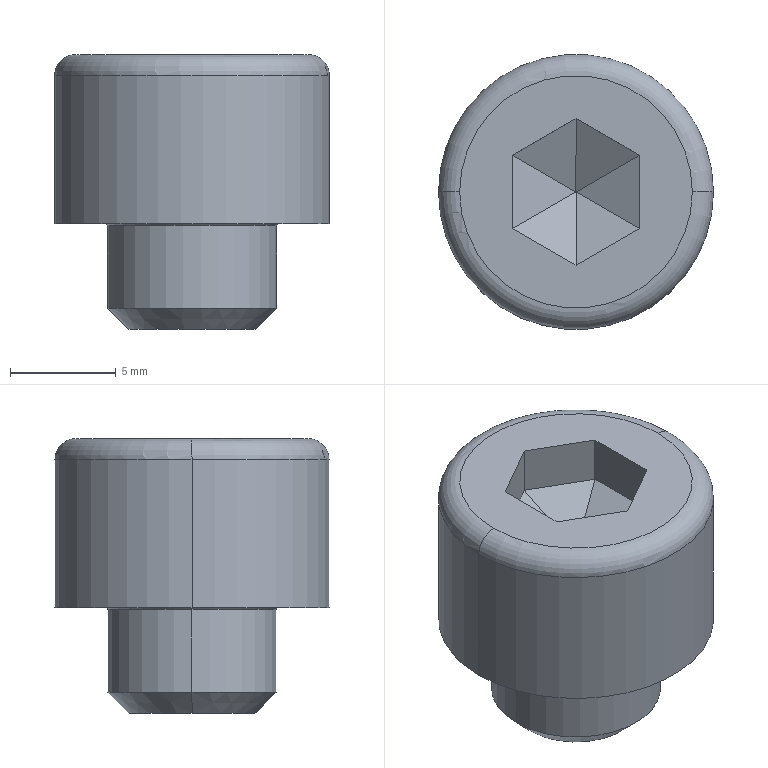Part | STEP file | Socket head cap screw M8x5 | 1 solid | 26 faces | box 13 x 13 x 13 mm | volume 1204 mm3 | plane 16 | torus 4 | cylinder 4 | cone 2 | commonest cylinder face diameters 8 x2 13 x2
STEP:
#1=CARTESIAN_POINT('',(-4.1,0.,0.));
#2=VERTEX_POINT('',#1);
#3=CARTESIAN_POINT('',(4.1,0.,0.));
#4=VERTEX_POINT('',#3);
#5=CARTESIAN_POINT('',(0.,0.,0.));
#6=DIRECTION('',(0.,0.,1.));
#7=DIRECTION('',(1.,0.,0.));
#8=AXIS2_PLACEMENT_3D('',#5,#6,#7);
#9=CIRCLE('',#8,4.1);
#10=EDGE_CURVE('',#2,#4,#9,.T.);
#11=ORIENTED_EDGE('',*,*,#10,.F.);
#12=CARTESIAN_POINT('',(-4.,0.,-0.1));
#13=VERTEX_POINT('',#12);
#14=CARTESIAN_POINT('',(-4.1,0.,-0.1));
#15=DIRECTION('',(0.,1.,0.));
#16=DIRECTION('',(-1.,0.,0.));
#17=AXIS2_PLACEMENT_3D('',#14,#15,#16);
#18=CIRCLE('',#17,0.1);
#19=EDGE_CURVE('',#2,#13,#18,.T.);
#20=ORIENTED_EDGE('',*,*,#19,.T.);
#21=CARTESIAN_POINT('',(4.,0.,-0.1));
#22=VERTEX_POINT('',#21);
#23=CARTESIAN_POINT('',(0.,0.,-0.1));
#24=DIRECTION('',(0.,0.,-1.));
#25=DIRECTION('',(1.,0.,0.));
#26=AXIS2_PLACEMENT_3D('',#23,#24,#25);
#27=CIRCLE('',#26,4.);
#28=EDGE_CURVE('',#22,#13,#27,.T.);
#29=ORIENTED_EDGE('',*,*,#28,.F.);
#30=CARTESIAN_POINT('',(4.1,0.,-0.1));
#31=DIRECTION('',(0.,-1.,0.));
#32=DIRECTION('',(0.,0.,-1.));
#33=AXIS2_PLACEMENT_3D('',#30,#31,#32);
#34=CIRCLE('',#33,0.1);
#35=EDGE_CURVE('',#4,#22,#34,.T.);
#36=ORIENTED_EDGE('',*,*,#35,.F.);
#37=EDGE_LOOP('',(#11,#20,#29,#36));
#38=FACE_OUTER_BOUND('',#37,.T.);
#39=CARTESIAN_POINT('',(0.,0.,-0.1));
#40=DIRECTION('',(0.,0.,1.));
#41=DIRECTION('',(1.,0.,0.));
#42=AXIS2_PLACEMENT_3D('',#39,#40,#41);
#43=TOROIDAL_SURFACE('',#42,4.1,0.1);
#44=ADVANCED_FACE('',(#38),#43,.F.);
#45=CARTESIAN_POINT('',(-6.5,0.,7.));
#46=VERTEX_POINT('',#45);
#47=CARTESIAN_POINT('',(6.5,0.,7.));
#48=VERTEX_POINT('',#47);
#49=CARTESIAN_POINT('',(0.,0.,7.));
#50=DIRECTION('',(0.,0.,-1.));
#51=DIRECTION('',(1.,0.,0.));
#52=AXIS2_PLACEMENT_3D('',#49,#50,#51);
#53=CIRCLE('',#52,6.5);
#54=EDGE_CURVE('',#46,#48,#53,.T.);
#55=ORIENTED_EDGE('',*,*,#54,.F.);
#56=CARTESIAN_POINT('',(-5.5,0.,8.));
#57=VERTEX_POINT('',#56);
#58=CARTESIAN_POINT('',(-5.5,0.,7.));
#59=DIRECTION('',(0.,1.,0.));
#60=DIRECTION('',(-1.,0.,0.));
#61=AXIS2_PLACEMENT_3D('',#58,#59,#60);
#62=CIRCLE('',#61,1.);
#63=EDGE_CURVE('',#46,#57,#62,.T.);
#64=ORIENTED_EDGE('',*,*,#63,.T.);
#65=CARTESIAN_POINT('',(5.5,0.,8.));
#66=VERTEX_POINT('',#65);
#67=CARTESIAN_POINT('',(0.,0.,8.));
#68=DIRECTION('',(0.,0.,1.));
#69=DIRECTION('',(1.,0.,0.));
#70=AXIS2_PLACEMENT_3D('',#67,#68,#69);
#71=CIRCLE('',#70,5.5);
#72=EDGE_CURVE('',#66,#57,#71,.T.);
#73=ORIENTED_EDGE('',*,*,#72,.F.);
#74=CARTESIAN_POINT('',(5.5,0.,7.));
#75=DIRECTION('',(0.,-1.,0.));
#76=DIRECTION('',(0.,0.,-1.));
#77=AXIS2_PLACEMENT_3D('',#74,#75,#76);
#78=CIRCLE('',#77,1.);
#79=EDGE_CURVE('',#48,#66,#78,.T.);
#80=ORIENTED_EDGE('',*,*,#79,.F.);
#81=EDGE_LOOP('',(#55,#64,#73,#80));
#82=FACE_OUTER_BOUND('',#81,.T.);
#83=CARTESIAN_POINT('',(0.,0.,7.));
#84=DIRECTION('',(0.,0.,1.));
#85=DIRECTION('',(1.,0.,0.));
#86=AXIS2_PLACEMENT_3D('',#83,#84,#85);
#87=TOROIDAL_SURFACE('',#86,5.5,1.);
#88=ADVANCED_FACE('',(#82),#87,.T.);
#89=CARTESIAN_POINT('',(-3.,0.,-5.));
#90=VERTEX_POINT('',#89);
#91=CARTESIAN_POINT('',(3.,0.,-5.));
#92=VERTEX_POINT('',#91);
#93=CARTESIAN_POINT('',(0.,0.,-5.));
#94=DIRECTION('',(0.,0.,-1.));
#95=DIRECTION('',(-1.,0.,0.));
#96=AXIS2_PLACEMENT_3D('',#93,#94,#95);
#97=CIRCLE('',#96,3.);
#98=EDGE_CURVE('',#90,#92,#97,.T.);
#99=ORIENTED_EDGE('',*,*,#98,.F.);
#100=CARTESIAN_POINT('',(-4.,0.,-4.));
#101=VERTEX_POINT('',#100);
#102=CARTESIAN_POINT('',(-3.,0.,-5.));
#103=DIRECTION('',(-0.7071,0.,0.7071));
#104=VECTOR('',#103,1000.);
#105=LINE('',#102,#104);
#106=EDGE_CURVE('',#90,#101,#105,.T.);
#107=ORIENTED_EDGE('',*,*,#106,.T.);
#108=CARTESIAN_POINT('',(4.,0.,-4.));
#109=VERTEX_POINT('',#108);
#110=CARTESIAN_POINT('',(0.,0.,-4.));
#111=DIRECTION('',(0.,0.,1.));
#112=DIRECTION('',(-1.,0.,0.));
#113=AXIS2_PLACEMENT_3D('',#110,#111,#112);
#114=CIRCLE('',#113,4.);
#115=EDGE_CURVE('',#109,#101,#114,.T.);
#116=ORIENTED_EDGE('',*,*,#115,.F.);
#117=CARTESIAN_POINT('',(3.,0.,-5.));
#118=DIRECTION('',(0.7071,0.,0.7071));
#119=VECTOR('',#118,1000.);
#120=LINE('',#117,#119);
#121=EDGE_CURVE('',#92,#109,#120,.T.);
#122=ORIENTED_EDGE('',*,*,#121,.F.);
#123=EDGE_LOOP('',(#99,#107,#116,#122));
#124=FACE_OUTER_BOUND('',#123,.T.);
#125=CARTESIAN_POINT('',(0.,0.,-5.));
#126=DIRECTION('',(0.,0.,1.));
#127=DIRECTION('',(1.,0.,0.));
#128=AXIS2_PLACEMENT_3D('',#125,#126,#127);
#129=CONICAL_SURFACE('',#128,3.,0.7854);
#130=ADVANCED_FACE('',(#124),#129,.T.);
#131=ORIENTED_EDGE('',*,*,#115,.T.);
#132=CARTESIAN_POINT('',(-4.,0.,-5.));
#133=DIRECTION('',(0.,0.,1.));
#134=VECTOR('',#133,1000.);
#135=LINE('',#132,#134);
#136=EDGE_CURVE('',#101,#13,#135,.T.);
#137=ORIENTED_EDGE('',*,*,#136,.T.);
#138=CARTESIAN_POINT('',(0.,0.,-0.1));
#139=DIRECTION('',(0.,0.,-1.));
#140=DIRECTION('',(1.,0.,0.));
#141=AXIS2_PLACEMENT_3D('',#138,#139,#140);
#142=CIRCLE('',#141,4.);
#143=EDGE_CURVE('',#13,#22,#142,.T.);
#144=ORIENTED_EDGE('',*,*,#143,.T.);
#145=CARTESIAN_POINT('',(4.,0.,-5.));
#146=DIRECTION('',(0.,0.,1.));
#147=VECTOR('',#146,1000.);
#148=LINE('',#145,#147);
#149=EDGE_CURVE('',#109,#22,#148,.T.);
#150=ORIENTED_EDGE('',*,*,#149,.F.);
#151=EDGE_LOOP('',(#131,#137,#144,#150));
#152=FACE_OUTER_BOUND('',#151,.T.);
#153=CARTESIAN_POINT('',(0.,0.,-5.));
#154=DIRECTION('',(0.,0.,1.));
#155=DIRECTION('',(1.,0.,0.));
#156=AXIS2_PLACEMENT_3D('',#153,#154,#155);
#157=CYLINDRICAL_SURFACE('',#156,4.);
#158=ADVANCED_FACE('',(#152),#157,.T.);
#159=ORIENTED_EDGE('',*,*,#54,.T.);
#160=CARTESIAN_POINT('',(6.5,0.,0.));
#161=VERTEX_POINT('',#160);
#162=CARTESIAN_POINT('',(6.5,0.,8.));
#163=DIRECTION('',(0.,0.,-1.));
#164=VECTOR('',#163,1000.);
#165=LINE('',#162,#164);
#166=EDGE_CURVE('',#48,#161,#165,.T.);
#167=ORIENTED_EDGE('',*,*,#166,.T.);
#168=CARTESIAN_POINT('',(-6.5,0.,0.));
#169=VERTEX_POINT('',#168);
#170=CARTESIAN_POINT('',(0.,0.,0.));
#171=DIRECTION('',(0.,0.,1.));
#172=DIRECTION('',(1.,0.,0.));
#173=AXIS2_PLACEMENT_3D('',#170,#171,#172);
#174=CIRCLE('',#173,6.5);
#175=EDGE_CURVE('',#161,#169,#174,.T.);
#176=ORIENTED_EDGE('',*,*,#175,.T.);
#177=CARTESIAN_POINT('',(-6.5,0.,8.));
#178=DIRECTION('',(0.,0.,-1.));
#179=VECTOR('',#178,1000.);
#180=LINE('',#177,#179);
#181=EDGE_CURVE('',#46,#169,#180,.T.);
#182=ORIENTED_EDGE('',*,*,#181,.F.);
#183=EDGE_LOOP('',(#159,#167,#176,#182));
#184=FACE_OUTER_BOUND('',#183,.T.);
#185=CARTESIAN_POINT('',(0.,0.,8.));
#186=DIRECTION('',(0.,0.,-1.));
#187=DIRECTION('',(-1.,0.,0.));
#188=AXIS2_PLACEMENT_3D('',#185,#186,#187);
#189=CYLINDRICAL_SURFACE('',#188,6.5);
#190=ADVANCED_FACE('',(#184),#189,.T.);
#191=CARTESIAN_POINT('',(0.,0.,0.));
#192=DIRECTION('',(0.,0.,1.));
#193=DIRECTION('',(1.,0.,0.));
#194=AXIS2_PLACEMENT_3D('',#191,#192,#193);
#195=CIRCLE('',#194,4.1);
#196=EDGE_CURVE('',#4,#2,#195,.T.);
#197=ORIENTED_EDGE('',*,*,#196,.T.);
#198=ORIENTED_EDGE('',*,*,#10,.T.);
#199=EDGE_LOOP('',(#197,#198));
#200=FACE_BOUND('',#199,.T.);
#201=CARTESIAN_POINT('',(0.,0.,0.));
#202=DIRECTION('',(0.,0.,1.));
#203=DIRECTION('',(1.,0.,0.));
#204=AXIS2_PLACEMENT_3D('',#201,#202,#203);
#205=CIRCLE('',#204,6.5);
#206=EDGE_CURVE('',#169,#161,#205,.T.);
#207=ORIENTED_EDGE('',*,*,#206,.F.);
#208=ORIENTED_EDGE('',*,*,#175,.F.);
#209=EDGE_LOOP('',(#207,#208));
#210=FACE_OUTER_BOUND('',#209,.T.);
#211=CARTESIAN_POINT('',(0.,0.,0.));
#212=DIRECTION('',(0.,0.,1.));
#213=DIRECTION('',(1.,0.,0.));
#214=AXIS2_PLACEMENT_3D('',#211,#212,#213);
#215=PLANE('',#214);
#216=ADVANCED_FACE('',(#200,#210),#215,.F.);
#217=ORIENTED_EDGE('',*,*,#166,.F.);
#218=CARTESIAN_POINT('',(0.,0.,7.));
#219=DIRECTION('',(0.,0.,-1.));
#220=DIRECTION('',(1.,0.,0.));
#221=AXIS2_PLACEMENT_3D('',#218,#219,#220);
#222=CIRCLE('',#221,6.5);
#223=EDGE_CURVE('',#48,#46,#222,.T.);
#224=ORIENTED_EDGE('',*,*,#223,.T.);
#225=ORIENTED_EDGE('',*,*,#181,.T.);
#226=ORIENTED_EDGE('',*,*,#206,.T.);
#227=EDGE_LOOP('',(#217,#224,#225,#226));
#228=FACE_OUTER_BOUND('',#227,.T.);
#229=CARTESIAN_POINT('',(0.,0.,8.));
#230=DIRECTION('',(0.,0.,-1.));
#231=DIRECTION('',(-1.,0.,0.));
#232=AXIS2_PLACEMENT_3D('',#229,#230,#231);
#233=CYLINDRICAL_SURFACE('',#232,6.5);
#234=ADVANCED_FACE('',(#228),#233,.T.);
#235=ORIENTED_EDGE('',*,*,#72,.T.);
#236=CARTESIAN_POINT('',(0.,0.,8.));
#237=DIRECTION('',(0.,0.,1.));
#238=DIRECTION('',(1.,0.,0.));
#239=AXIS2_PLACEMENT_3D('',#236,#237,#238);
#240=CIRCLE('',#239,5.5);
#241=EDGE_CURVE('',#57,#66,#240,.T.);
#242=ORIENTED_EDGE('',*,*,#241,.T.);
#243=EDGE_LOOP('',(#235,#242));
#244=FACE_OUTER_BOUND('',#243,.T.);
#245=CARTESIAN_POINT('',(3.,-1.732,8.));
#246=VERTEX_POINT('',#245);
#247=CARTESIAN_POINT('',(3.,1.732,8.));
#248=VERTEX_POINT('',#247);
#249=CARTESIAN_POINT('',(3.,-1.732,8.));
#250=DIRECTION('',(0.,1.,0.));
#251=VECTOR('',#250,1000.);
#252=LINE('',#249,#251);
#253=EDGE_CURVE('',#246,#248,#252,.T.);
#254=ORIENTED_EDGE('',*,*,#253,.F.);
#255=CARTESIAN_POINT('',(0.,-3.464,8.));
#256=VERTEX_POINT('',#255);
#257=CARTESIAN_POINT('',(0.,-3.464,8.));
#258=DIRECTION('',(0.866,0.5,0.));
#259=VECTOR('',#258,1000.);
#260=LINE('',#257,#259);
#261=EDGE_CURVE('',#256,#246,#260,.T.);
#262=ORIENTED_EDGE('',*,*,#261,.F.);
#263=CARTESIAN_POINT('',(-3.,-1.732,8.));
#264=VERTEX_POINT('',#263);
#265=CARTESIAN_POINT('',(-3.,-1.732,8.));
#266=DIRECTION('',(0.866,-0.5,0.));
#267=VECTOR('',#266,1000.);
#268=LINE('',#265,#267);
#269=EDGE_CURVE('',#264,#256,#268,.T.);
#270=ORIENTED_EDGE('',*,*,#269,.F.);
#271=CARTESIAN_POINT('',(-3.,1.732,8.));
#272=VERTEX_POINT('',#271);
#273=CARTESIAN_POINT('',(-3.,1.732,8.));
#274=DIRECTION('',(0.,-1.,0.));
#275=VECTOR('',#274,1000.);
#276=LINE('',#273,#275);
#277=EDGE_CURVE('',#272,#264,#276,.T.);
#278=ORIENTED_EDGE('',*,*,#277,.F.);
#279=CARTESIAN_POINT('',(0.,3.464,8.));
#280=VERTEX_POINT('',#279);
#281=CARTESIAN_POINT('',(0.,3.464,8.));
#282=DIRECTION('',(-0.866,-0.5,0.));
#283=VECTOR('',#282,1000.);
#284=LINE('',#281,#283);
#285=EDGE_CURVE('',#280,#272,#284,.T.);
#286=ORIENTED_EDGE('',*,*,#285,.F.);
#287=CARTESIAN_POINT('',(3.,1.732,8.));
#288=DIRECTION('',(-0.866,0.5,0.));
#289=VECTOR('',#288,1000.);
#290=LINE('',#287,#289);
#291=EDGE_CURVE('',#248,#280,#290,.T.);
#292=ORIENTED_EDGE('',*,*,#291,.F.);
#293=EDGE_LOOP('',(#254,#262,#270,#278,#286,#292));
#294=FACE_BOUND('',#293,.T.);
#295=CARTESIAN_POINT('',(0.,0.,8.));
#296=DIRECTION('',(0.,0.,1.));
#297=DIRECTION('',(1.,0.,0.));
#298=AXIS2_PLACEMENT_3D('',#295,#296,#297);
#299=PLANE('',#298);
#300=ADVANCED_FACE('',(#244,#294),#299,.T.);
#301=CARTESIAN_POINT('',(3.,1.732,5.729));
#302=VERTEX_POINT('',#301);
#303=CARTESIAN_POINT('',(3.,1.732,4.));
#304=DIRECTION('',(0.,0.,1.));
#305=VECTOR('',#304,1000.);
#306=LINE('',#303,#305);
#307=EDGE_CURVE('',#302,#248,#306,.T.);
#308=ORIENTED_EDGE('',*,*,#307,.F.);
#309=CARTESIAN_POINT('',(3.,-1.732,5.729));
#310=VERTEX_POINT('',#309);
#311=CARTESIAN_POINT('',(3.,-1.732,5.729));
#312=DIRECTION('',(0.,-1.,0.));
#313=VECTOR('',#312,1000.);
#314=LINE('',#311,#313);
#315=EDGE_CURVE('',#302,#310,#314,.T.);
#316=ORIENTED_EDGE('',*,*,#315,.T.);
#317=CARTESIAN_POINT('',(3.,-1.732,4.));
#318=DIRECTION('',(0.,0.,1.));
#319=VECTOR('',#318,1000.);
#320=LINE('',#317,#319);
#321=EDGE_CURVE('',#310,#246,#320,.T.);
#322=ORIENTED_EDGE('',*,*,#321,.T.);
#323=ORIENTED_EDGE('',*,*,#253,.T.);
#324=EDGE_LOOP('',(#308,#316,#322,#323));
#325=FACE_OUTER_BOUND('',#324,.T.);
#326=CARTESIAN_POINT('',(3.,-1.732,4.));
#327=DIRECTION('',(1.,0.,0.));
#328=DIRECTION('',(0.,1.,0.));
#329=AXIS2_PLACEMENT_3D('',#326,#327,#328);
#330=PLANE('',#329);
#331=ADVANCED_FACE('',(#325),#330,.F.);
#332=ORIENTED_EDGE('',*,*,#321,.F.);
#333=CARTESIAN_POINT('',(0.,-3.464,5.729));
#334=VERTEX_POINT('',#333);
#335=CARTESIAN_POINT('',(0.,-3.464,5.729));
#336=DIRECTION('',(-0.866,-0.5,0.));
#337=VECTOR('',#336,1000.);
#338=LINE('',#335,#337);
#339=EDGE_CURVE('',#310,#334,#338,.T.);
#340=ORIENTED_EDGE('',*,*,#339,.T.);
#341=CARTESIAN_POINT('',(0.,-3.464,4.));
#342=DIRECTION('',(0.,0.,1.));
#343=VECTOR('',#342,1000.);
#344=LINE('',#341,#343);
#345=EDGE_CURVE('',#334,#256,#344,.T.);
#346=ORIENTED_EDGE('',*,*,#345,.T.);
#347=ORIENTED_EDGE('',*,*,#261,.T.);
#348=EDGE_LOOP('',(#332,#340,#346,#347));
#349=FACE_OUTER_BOUND('',#348,.T.);
#350=CARTESIAN_POINT('',(0.,-3.464,4.));
#351=DIRECTION('',(0.5,-0.866,0.));
#352=DIRECTION('',(0.866,0.5,0.));
#353=AXIS2_PLACEMENT_3D('',#350,#351,#352);
#354=PLANE('',#353);
#355=ADVANCED_FACE('',(#349),#354,.F.);
#356=ORIENTED_EDGE('',*,*,#345,.F.);
#357=CARTESIAN_POINT('',(-3.,-1.732,5.729));
#358=VERTEX_POINT('',#357);
#359=CARTESIAN_POINT('',(-3.,-1.732,5.729));
#360=DIRECTION('',(-0.866,0.5,0.));
#361=VECTOR('',#360,1000.);
#362=LINE('',#359,#361);
#363=EDGE_CURVE('',#334,#358,#362,.T.);
#364=ORIENTED_EDGE('',*,*,#363,.T.);
#365=CARTESIAN_POINT('',(-3.,-1.732,4.));
#366=DIRECTION('',(0.,0.,1.));
#367=VECTOR('',#366,1000.);
#368=LINE('',#365,#367);
#369=EDGE_CURVE('',#358,#264,#368,.T.);
#370=ORIENTED_EDGE('',*,*,#369,.T.);
#371=ORIENTED_EDGE('',*,*,#269,.T.);
#372=EDGE_LOOP('',(#356,#364,#370,#371));
#373=FACE_OUTER_BOUND('',#372,.T.);
#374=CARTESIAN_POINT('',(-3.,-1.732,4.));
#375=DIRECTION('',(-0.5,-0.866,0.));
#376=DIRECTION('',(0.866,-0.5,0.));
#377=AXIS2_PLACEMENT_3D('',#374,#375,#376);
#378=PLANE('',#377);
#379=ADVANCED_FACE('',(#373),#378,.F.);
#380=ORIENTED_EDGE('',*,*,#369,.F.);
#381=CARTESIAN_POINT('',(-3.,1.732,5.729));
#382=VERTEX_POINT('',#381);
#383=CARTESIAN_POINT('',(-3.,1.732,5.729));
#384=DIRECTION('',(0.,1.,0.));
#385=VECTOR('',#384,1000.);
#386=LINE('',#383,#385);
#387=EDGE_CURVE('',#358,#382,#386,.T.);
#388=ORIENTED_EDGE('',*,*,#387,.T.);
#389=CARTESIAN_POINT('',(-3.,1.732,4.));
#390=DIRECTION('',(0.,0.,1.));
#391=VECTOR('',#390,1000.);
#392=LINE('',#389,#391);
#393=EDGE_CURVE('',#382,#272,#392,.T.);
#394=ORIENTED_EDGE('',*,*,#393,.T.);
#395=ORIENTED_EDGE('',*,*,#277,.T.);
#396=EDGE_LOOP('',(#380,#388,#394,#395));
#397=FACE_OUTER_BOUND('',#396,.T.);
#398=CARTESIAN_POINT('',(-3.,1.732,4.));
#399=DIRECTION('',(-1.,0.,0.));
#400=DIRECTION('',(0.,0.,1.));
#401=AXIS2_PLACEMENT_3D('',#398,#399,#400);
#402=PLANE('',#401);
#403=ADVANCED_FACE('',(#397),#402,.F.);
#404=ORIENTED_EDGE('',*,*,#393,.F.);
#405=CARTESIAN_POINT('',(0.,3.464,5.729));
#406=VERTEX_POINT('',#405);
#407=CARTESIAN_POINT('',(0.,3.464,5.729));
#408=DIRECTION('',(0.866,0.5,0.));
#409=VECTOR('',#408,1000.);
#410=LINE('',#407,#409);
#411=EDGE_CURVE('',#382,#406,#410,.T.);
#412=ORIENTED_EDGE('',*,*,#411,.T.);
#413=CARTESIAN_POINT('',(0.,3.464,4.));
#414=DIRECTION('',(0.,0.,1.));
#415=VECTOR('',#414,1000.);
#416=LINE('',#413,#415);
#417=EDGE_CURVE('',#406,#280,#416,.T.);
#418=ORIENTED_EDGE('',*,*,#417,.T.);
#419=ORIENTED_EDGE('',*,*,#285,.T.);
#420=EDGE_LOOP('',(#404,#412,#418,#419));
#421=FACE_OUTER_BOUND('',#420,.T.);
#422=CARTESIAN_POINT('',(0.,3.464,4.));
#423=DIRECTION('',(-0.5,0.866,0.));
#424=DIRECTION('',(-0.866,-0.5,0.));
#425=AXIS2_PLACEMENT_3D('',#422,#423,#424);
#426=PLANE('',#425);
#427=ADVANCED_FACE('',(#421),#426,.F.);
#428=ORIENTED_EDGE('',*,*,#417,.F.);
#429=CARTESIAN_POINT('',(3.,1.732,5.729));
#430=DIRECTION('',(0.866,-0.5,0.));
#431=VECTOR('',#430,1000.);
#432=LINE('',#429,#431);
#433=EDGE_CURVE('',#406,#302,#432,.T.);
#434=ORIENTED_EDGE('',*,*,#433,.T.);
#435=ORIENTED_EDGE('',*,*,#307,.T.);
#436=ORIENTED_EDGE('',*,*,#291,.T.);
#437=EDGE_LOOP('',(#428,#434,#435,#436));
#438=FACE_OUTER_BOUND('',#437,.T.);
#439=CARTESIAN_POINT('',(3.,1.732,4.));
#440=DIRECTION('',(0.5,0.866,0.));
#441=DIRECTION('',(-0.866,0.5,0.));
#442=AXIS2_PLACEMENT_3D('',#439,#440,#441);
#443=PLANE('',#442);
#444=ADVANCED_FACE('',(#438),#443,.F.);
#445=CARTESIAN_POINT('',(0.,0.005888,4.));
#446=VERTEX_POINT('',#445);
#447=CARTESIAN_POINT('',(-0.005099,0.002944,4.));
#448=VERTEX_POINT('',#447);
#449=CARTESIAN_POINT('',(-0.00255,0.004416,4.));
#450=DIRECTION('',(-0.866,-0.5,0.));
#451=VECTOR('',#450,1000.);
#452=LINE('',#449,#451);
#453=EDGE_CURVE('',#446,#448,#452,.T.);
#454=ORIENTED_EDGE('',*,*,#453,.T.);
#455=CARTESIAN_POINT('',(-0.005099,-0.002944,4.));
#456=VERTEX_POINT('',#455);
#457=CARTESIAN_POINT('',(-0.005099,0.,4.));
#458=DIRECTION('',(0.,-1.,0.));
#459=VECTOR('',#458,1000.);
#460=LINE('',#457,#459);
#461=EDGE_CURVE('',#448,#456,#460,.T.);
#462=ORIENTED_EDGE('',*,*,#461,.T.);
#463=CARTESIAN_POINT('',(0.,-0.005888,4.));
#464=VERTEX_POINT('',#463);
#465=CARTESIAN_POINT('',(-0.00255,-0.004416,4.));
#466=DIRECTION('',(0.866,-0.5,0.));
#467=VECTOR('',#466,1000.);
#468=LINE('',#465,#467);
#469=EDGE_CURVE('',#456,#464,#468,.T.);
#470=ORIENTED_EDGE('',*,*,#469,.T.);
#471=CARTESIAN_POINT('',(0.005099,-0.002944,4.));
#472=VERTEX_POINT('',#471);
#473=CARTESIAN_POINT('',(0.00255,-0.004416,4.));
#474=DIRECTION('',(0.866,0.5,0.));
#475=VECTOR('',#474,1000.);
#476=LINE('',#473,#475);
#477=EDGE_CURVE('',#464,#472,#476,.T.);
#478=ORIENTED_EDGE('',*,*,#477,.T.);
#479=CARTESIAN_POINT('',(0.005099,0.002944,4.));
#480=VERTEX_POINT('',#479);
#481=CARTESIAN_POINT('',(0.005099,0.,4.));
#482=DIRECTION('',(0.,1.,0.));
#483=VECTOR('',#482,1000.);
#484=LINE('',#481,#483);
#485=EDGE_CURVE('',#472,#480,#484,.T.);
#486=ORIENTED_EDGE('',*,*,#485,.T.);
#487=CARTESIAN_POINT('',(0.00255,0.004416,4.));
#488=DIRECTION('',(-0.866,0.5,0.));
#489=VECTOR('',#488,1000.);
#490=LINE('',#487,#489);
#491=EDGE_CURVE('',#480,#446,#490,.T.);
#492=ORIENTED_EDGE('',*,*,#491,.T.);
#493=EDGE_LOOP('',(#454,#462,#470,#478,#486,#492));
#494=FACE_OUTER_BOUND('',#493,.T.);
#495=CARTESIAN_POINT('',(0.,0.,4.));
#496=DIRECTION('',(0.,0.,1.));
#497=DIRECTION('',(1.,0.,0.));
#498=AXIS2_PLACEMENT_3D('',#495,#496,#497);
#499=PLANE('',#498);
#500=ADVANCED_FACE('',(#494),#499,.T.);
#501=ORIENTED_EDGE('',*,*,#136,.F.);
#502=CARTESIAN_POINT('',(0.,0.,-4.));
#503=DIRECTION('',(0.,0.,1.));
#504=DIRECTION('',(-1.,0.,0.));
#505=AXIS2_PLACEMENT_3D('',#502,#503,#504);
#506=CIRCLE('',#505,4.);
#507=EDGE_CURVE('',#101,#109,#506,.T.);
#508=ORIENTED_EDGE('',*,*,#507,.T.);
#509=ORIENTED_EDGE('',*,*,#149,.T.);
#510=ORIENTED_EDGE('',*,*,#28,.T.);
#511=EDGE_LOOP('',(#501,#508,#509,#510));
#512=FACE_OUTER_BOUND('',#511,.T.);
#513=CARTESIAN_POINT('',(0.,0.,-5.));
#514=DIRECTION('',(0.,0.,1.));
#515=DIRECTION('',(1.,0.,0.));
#516=AXIS2_PLACEMENT_3D('',#513,#514,#515);
#517=CYLINDRICAL_SURFACE('',#516,4.);
#518=ADVANCED_FACE('',(#512),#517,.T.);
#519=CARTESIAN_POINT('',(0.,0.,-5.));
#520=DIRECTION('',(0.,0.,-1.));
#521=DIRECTION('',(-1.,0.,0.));
#522=AXIS2_PLACEMENT_3D('',#519,#520,#521);
#523=CIRCLE('',#522,3.);
#524=EDGE_CURVE('',#92,#90,#523,.T.);
#525=ORIENTED_EDGE('',*,*,#524,.T.);
#526=ORIENTED_EDGE('',*,*,#98,.T.);
#527=EDGE_LOOP('',(#525,#526));
#528=FACE_OUTER_BOUND('',#527,.T.);
#529=CARTESIAN_POINT('',(0.,0.,-5.));
#530=DIRECTION('',(0.,0.,-1.));
#531=DIRECTION('',(-1.,0.,0.));
#532=AXIS2_PLACEMENT_3D('',#529,#530,#531);
#533=PLANE('',#532);
#534=ADVANCED_FACE('',(#528),#533,.T.);
#535=ORIENTED_EDGE('',*,*,#106,.F.);
#536=ORIENTED_EDGE('',*,*,#524,.F.);
#537=ORIENTED_EDGE('',*,*,#121,.T.);
#538=ORIENTED_EDGE('',*,*,#507,.F.);
#539=EDGE_LOOP('',(#535,#536,#537,#538));
#540=FACE_OUTER_BOUND('',#539,.T.);
#541=CARTESIAN_POINT('',(0.,0.,-5.));
#542=DIRECTION('',(0.,0.,1.));
#543=DIRECTION('',(1.,0.,0.));
#544=AXIS2_PLACEMENT_3D('',#541,#542,#543);
#545=CONICAL_SURFACE('',#544,3.,0.7854);
#546=ADVANCED_FACE('',(#540),#545,.T.);
#547=ORIENTED_EDGE('',*,*,#63,.F.);
#548=ORIENTED_EDGE('',*,*,#223,.F.);
#549=ORIENTED_EDGE('',*,*,#79,.T.);
#550=ORIENTED_EDGE('',*,*,#241,.F.);
#551=EDGE_LOOP('',(#547,#548,#549,#550));
#552=FACE_OUTER_BOUND('',#551,.T.);
#553=CARTESIAN_POINT('',(0.,0.,7.));
#554=DIRECTION('',(0.,0.,1.));
#555=DIRECTION('',(1.,0.,0.));
#556=AXIS2_PLACEMENT_3D('',#553,#554,#555);
#557=TOROIDAL_SURFACE('',#556,5.5,1.);
#558=ADVANCED_FACE('',(#552),#557,.T.);
#559=CARTESIAN_POINT('',(0.00408,-0.002355,3.999));
#560=DIRECTION('',(-0.7746,0.4472,-0.4472));
#561=VECTOR('',#560,1000.);
#562=LINE('',#559,#561);
#563=EDGE_CURVE('',#310,#472,#562,.T.);
#564=ORIENTED_EDGE('',*,*,#563,.F.);
#565=ORIENTED_EDGE('',*,*,#315,.F.);
#566=CARTESIAN_POINT('',(0.00408,0.002355,3.999));
#567=DIRECTION('',(0.7746,0.4472,0.4472));
#568=VECTOR('',#567,1000.);
#569=LINE('',#566,#568);
#570=EDGE_CURVE('',#480,#302,#569,.T.);
#571=ORIENTED_EDGE('',*,*,#570,.F.);
#572=ORIENTED_EDGE('',*,*,#485,.F.);
#573=EDGE_LOOP('',(#564,#565,#571,#572));
#574=FACE_OUTER_BOUND('',#573,.T.);
#575=CARTESIAN_POINT('',(0.005099,0.,4.));
#576=DIRECTION('',(0.5,0.,-0.866));
#577=DIRECTION('',(0.,1.,0.));
#578=AXIS2_PLACEMENT_3D('',#575,#576,#577);
#579=PLANE('',#578);
#580=ADVANCED_FACE('',(#574),#579,.F.);
#581=ORIENTED_EDGE('',*,*,#570,.T.);
#582=ORIENTED_EDGE('',*,*,#433,.F.);
#583=CARTESIAN_POINT('',(0.,0.004711,3.999));
#584=DIRECTION('',(0.,0.8944,0.4472));
#585=VECTOR('',#584,1000.);
#586=LINE('',#583,#585);
#587=EDGE_CURVE('',#446,#406,#586,.T.);
#588=ORIENTED_EDGE('',*,*,#587,.F.);
#589=ORIENTED_EDGE('',*,*,#491,.F.);
#590=EDGE_LOOP('',(#581,#582,#588,#589));
#591=FACE_OUTER_BOUND('',#590,.T.);
#592=CARTESIAN_POINT('',(0.00255,0.004416,4.));
#593=DIRECTION('',(0.25,0.433,-0.866));
#594=DIRECTION('',(-0.866,0.5,0.));
#595=AXIS2_PLACEMENT_3D('',#592,#593,#594);
#596=PLANE('',#595);
#597=ADVANCED_FACE('',(#591),#596,.F.);
#598=ORIENTED_EDGE('',*,*,#563,.T.);
#599=ORIENTED_EDGE('',*,*,#477,.F.);
#600=CARTESIAN_POINT('',(0.,-0.004711,3.999));
#601=DIRECTION('',(0.,0.8944,-0.4472));
#602=VECTOR('',#601,1000.);
#603=LINE('',#600,#602);
#604=EDGE_CURVE('',#334,#464,#603,.T.);
#605=ORIENTED_EDGE('',*,*,#604,.F.);
#606=ORIENTED_EDGE('',*,*,#339,.F.);
#607=EDGE_LOOP('',(#598,#599,#605,#606));
#608=FACE_OUTER_BOUND('',#607,.T.);
#609=CARTESIAN_POINT('',(0.00255,-0.004416,4.));
#610=DIRECTION('',(0.25,-0.433,-0.866));
#611=DIRECTION('',(0.866,0.5,0.));
#612=AXIS2_PLACEMENT_3D('',#609,#610,#611);
#613=PLANE('',#612);
#614=ADVANCED_FACE('',(#608),#613,.F.);
#615=ORIENTED_EDGE('',*,*,#587,.T.);
#616=ORIENTED_EDGE('',*,*,#411,.F.);
#617=CARTESIAN_POINT('',(-0.00408,0.002355,3.999));
#618=DIRECTION('',(-0.7746,0.4472,0.4472));
#619=VECTOR('',#618,1000.);
#620=LINE('',#617,#619);
#621=EDGE_CURVE('',#448,#382,#620,.T.);
#622=ORIENTED_EDGE('',*,*,#621,.F.);
#623=ORIENTED_EDGE('',*,*,#453,.F.);
#624=EDGE_LOOP('',(#615,#616,#622,#623));
#625=FACE_OUTER_BOUND('',#624,.T.);
#626=CARTESIAN_POINT('',(-0.00255,0.004416,4.));
#627=DIRECTION('',(-0.25,0.433,-0.866));
#628=DIRECTION('',(-0.866,-0.5,0.));
#629=AXIS2_PLACEMENT_3D('',#626,#627,#628);
#630=PLANE('',#629);
#631=ADVANCED_FACE('',(#625),#630,.F.);
#632=ORIENTED_EDGE('',*,*,#604,.T.);
#633=ORIENTED_EDGE('',*,*,#469,.F.);
#634=CARTESIAN_POINT('',(-0.00408,-0.002355,3.999));
#635=DIRECTION('',(0.7746,0.4472,-0.4472));
#636=VECTOR('',#635,1000.);
#637=LINE('',#634,#636);
#638=EDGE_CURVE('',#358,#456,#637,.T.);
#639=ORIENTED_EDGE('',*,*,#638,.F.);
#640=ORIENTED_EDGE('',*,*,#363,.F.);
#641=EDGE_LOOP('',(#632,#633,#639,#640));
#642=FACE_OUTER_BOUND('',#641,.T.);
#643=CARTESIAN_POINT('',(-0.00255,-0.004416,4.));
#644=DIRECTION('',(-0.25,-0.433,-0.866));
#645=DIRECTION('',(0.866,-0.5,0.));
#646=AXIS2_PLACEMENT_3D('',#643,#644,#645);
#647=PLANE('',#646);
#648=ADVANCED_FACE('',(#642),#647,.F.);
#649=ORIENTED_EDGE('',*,*,#621,.T.);
#650=ORIENTED_EDGE('',*,*,#387,.F.);
#651=ORIENTED_EDGE('',*,*,#638,.T.);
#652=ORIENTED_EDGE('',*,*,#461,.F.);
#653=EDGE_LOOP('',(#649,#650,#651,#652));
#654=FACE_OUTER_BOUND('',#653,.T.);
#655=CARTESIAN_POINT('',(-0.005099,0.,4.));
#656=DIRECTION('',(-0.5,0.,-0.866));
#657=DIRECTION('',(0.,-1.,0.));
#658=AXIS2_PLACEMENT_3D('',#655,#656,#657);
#659=PLANE('',#658);
#660=ADVANCED_FACE('',(#654),#659,.F.);
#661=ORIENTED_EDGE('',*,*,#19,.F.);
#662=ORIENTED_EDGE('',*,*,#196,.F.);
#663=ORIENTED_EDGE('',*,*,#35,.T.);
#664=ORIENTED_EDGE('',*,*,#143,.F.);
#665=EDGE_LOOP('',(#661,#662,#663,#664));
#666=FACE_OUTER_BOUND('',#665,.T.);
#667=CARTESIAN_POINT('',(0.,0.,-0.1));
#668=DIRECTION('',(0.,0.,1.));
#669=DIRECTION('',(1.,0.,0.));
#670=AXIS2_PLACEMENT_3D('',#667,#668,#669);
#671=TOROIDAL_SURFACE('',#670,4.1,0.1);
#672=ADVANCED_FACE('',(#666),#671,.F.);
#673=CLOSED_SHELL('',(#44,#88,#130,#158,#190,#216,#234,#300,#331,#355,#379,#403,#427,#444,#500,#518,#534,#546,#558,#580,#597,#614,#631,#648,#660,#672));
#674=MANIFOLD_SOLID_BREP('',#673);
#675=CARTESIAN_POINT('',(0.,0.,0.));
#676=DIRECTION('',(0.,0.,1.));
#677=DIRECTION('',(1.,0.,0.));
#678=AXIS2_PLACEMENT_3D('',#675,#676,#677);
#679=(LENGTH_UNIT()NAMED_UNIT(*)SI_UNIT(.MILLI.,.METRE.));
#680=UNCERTAINTY_MEASURE_WITH_UNIT(LENGTH_MEASURE(0.00001),#679,'','');
#681=(NAMED_UNIT(*)PLANE_ANGLE_UNIT()SI_UNIT($,.RADIAN.));
#682=(NAMED_UNIT(*)SI_UNIT($,.STERADIAN.)SOLID_ANGLE_UNIT());
#683=(GEOMETRIC_REPRESENTATION_CONTEXT(3)GLOBAL_UNCERTAINTY_ASSIGNED_CONTEXT((#680))GLOBAL_UNIT_ASSIGNED_CONTEXT((#679,#681,#682))REPRESENTATION_CONTEXT('',''));
#684=ADVANCED_BREP_SHAPE_REPRESENTATION('',(#674,#678),#683);